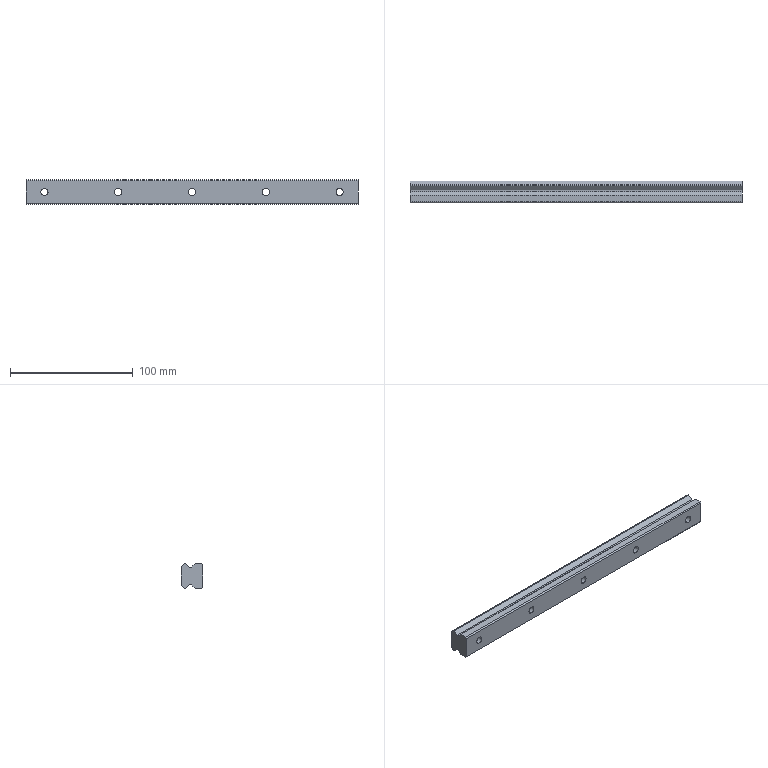Part | SolidWorks | features BaseBody 1 | 1 solid | 43 faces | box 270 x 17.5 x 20 mm | volume 81053 mm3 | plane 23 | cylinder 20 | commonest cylinder face diameters 5.8 x10 9.5 x10
STEP:
#1=CARTESIAN_POINT('',(64.75,9.,0.));
#2=VERTEX_POINT('',#1);
#3=CARTESIAN_POINT('',(55.25,9.,0.));
#4=VERTEX_POINT('',#3);
#5=CARTESIAN_POINT('',(60.,9.,0.));
#6=DIRECTION('',(0.,-1.,0.));
#7=DIRECTION('',(1.,0.,0.));
#8=AXIS2_PLACEMENT_3D('',#5,#6,#7);
#9=CIRCLE('',#8,4.75);
#10=EDGE_CURVE('',#2,#4,#9,.T.);
#11=ORIENTED_EDGE('',*,*,#10,.T.);
#12=CARTESIAN_POINT('',(55.25,17.5,0.));
#13=VERTEX_POINT('',#12);
#14=CARTESIAN_POINT('',(55.25,0.,0.));
#15=DIRECTION('',(0.,1.,0.));
#16=VECTOR('',#15,1000.);
#17=LINE('',#14,#16);
#18=EDGE_CURVE('',#4,#13,#17,.T.);
#19=ORIENTED_EDGE('',*,*,#18,.T.);
#20=CARTESIAN_POINT('',(64.75,17.5,0.));
#21=VERTEX_POINT('',#20);
#22=CARTESIAN_POINT('',(60.,17.5,0.));
#23=DIRECTION('',(0.,-1.,0.));
#24=DIRECTION('',(1.,0.,0.));
#25=AXIS2_PLACEMENT_3D('',#22,#23,#24);
#26=CIRCLE('',#25,4.75);
#27=EDGE_CURVE('',#21,#13,#26,.T.);
#28=ORIENTED_EDGE('',*,*,#27,.F.);
#29=CARTESIAN_POINT('',(64.75,0.,0.));
#30=DIRECTION('',(0.,1.,0.));
#31=VECTOR('',#30,1000.);
#32=LINE('',#29,#31);
#33=EDGE_CURVE('',#2,#21,#32,.T.);
#34=ORIENTED_EDGE('',*,*,#33,.F.);
#35=EDGE_LOOP('',(#11,#19,#28,#34));
#36=FACE_OUTER_BOUND('',#35,.T.);
#37=CARTESIAN_POINT('',(60.,0.,0.));
#38=DIRECTION('',(0.,1.,0.));
#39=DIRECTION('',(1.,0.,0.));
#40=AXIS2_PLACEMENT_3D('',#37,#38,#39);
#41=CYLINDRICAL_SURFACE('',#40,4.75);
#42=ADVANCED_FACE('',(#36),#41,.F.);
#43=CARTESIAN_POINT('',(62.9,0.,0.));
#44=VERTEX_POINT('',#43);
#45=CARTESIAN_POINT('',(57.1,0.,0.));
#46=VERTEX_POINT('',#45);
#47=CARTESIAN_POINT('',(60.,0.,0.));
#48=DIRECTION('',(0.,-1.,0.));
#49=DIRECTION('',(1.,0.,0.));
#50=AXIS2_PLACEMENT_3D('',#47,#48,#49);
#51=CIRCLE('',#50,2.9);
#52=EDGE_CURVE('',#44,#46,#51,.T.);
#53=ORIENTED_EDGE('',*,*,#52,.T.);
#54=CARTESIAN_POINT('',(57.1,9.,0.));
#55=VERTEX_POINT('',#54);
#56=CARTESIAN_POINT('',(57.1,0.,0.));
#57=DIRECTION('',(0.,1.,0.));
#58=VECTOR('',#57,1000.);
#59=LINE('',#56,#58);
#60=EDGE_CURVE('',#46,#55,#59,.T.);
#61=ORIENTED_EDGE('',*,*,#60,.T.);
#62=CARTESIAN_POINT('',(62.9,9.,0.));
#63=VERTEX_POINT('',#62);
#64=CARTESIAN_POINT('',(60.,9.,0.));
#65=DIRECTION('',(0.,-1.,0.));
#66=DIRECTION('',(1.,0.,0.));
#67=AXIS2_PLACEMENT_3D('',#64,#65,#66);
#68=CIRCLE('',#67,2.9);
#69=EDGE_CURVE('',#63,#55,#68,.T.);
#70=ORIENTED_EDGE('',*,*,#69,.F.);
#71=CARTESIAN_POINT('',(62.9,0.,0.));
#72=DIRECTION('',(0.,1.,0.));
#73=VECTOR('',#72,1000.);
#74=LINE('',#71,#73);
#75=EDGE_CURVE('',#44,#63,#74,.T.);
#76=ORIENTED_EDGE('',*,*,#75,.F.);
#77=EDGE_LOOP('',(#53,#61,#70,#76));
#78=FACE_OUTER_BOUND('',#77,.T.);
#79=CARTESIAN_POINT('',(60.,0.,0.));
#80=DIRECTION('',(0.,1.,0.));
#81=DIRECTION('',(1.,0.,0.));
#82=AXIS2_PLACEMENT_3D('',#79,#80,#81);
#83=CYLINDRICAL_SURFACE('',#82,2.9);
#84=ADVANCED_FACE('',(#78),#83,.F.);
#85=CARTESIAN_POINT('',(120.,9.,-4.75));
#86=VERTEX_POINT('',#85);
#87=CARTESIAN_POINT('',(120.,9.,4.75));
#88=VERTEX_POINT('',#87);
#89=CARTESIAN_POINT('',(120.,9.,0.));
#90=DIRECTION('',(0.,-1.,0.));
#91=DIRECTION('',(0.,0.,-1.));
#92=AXIS2_PLACEMENT_3D('',#89,#90,#91);
#93=CIRCLE('',#92,4.75);
#94=EDGE_CURVE('',#86,#88,#93,.T.);
#95=ORIENTED_EDGE('',*,*,#94,.T.);
#96=CARTESIAN_POINT('',(120.,17.5,4.75));
#97=VERTEX_POINT('',#96);
#98=CARTESIAN_POINT('',(120.,0.,4.75));
#99=DIRECTION('',(0.,1.,0.));
#100=VECTOR('',#99,1000.);
#101=LINE('',#98,#100);
#102=EDGE_CURVE('',#88,#97,#101,.T.);
#103=ORIENTED_EDGE('',*,*,#102,.T.);
#104=CARTESIAN_POINT('',(120.,17.5,-4.75));
#105=VERTEX_POINT('',#104);
#106=CARTESIAN_POINT('',(120.,17.5,0.));
#107=DIRECTION('',(0.,-1.,0.));
#108=DIRECTION('',(0.,0.,-1.));
#109=AXIS2_PLACEMENT_3D('',#106,#107,#108);
#110=CIRCLE('',#109,4.75);
#111=EDGE_CURVE('',#105,#97,#110,.T.);
#112=ORIENTED_EDGE('',*,*,#111,.F.);
#113=CARTESIAN_POINT('',(120.,0.,-4.75));
#114=DIRECTION('',(0.,1.,0.));
#115=VECTOR('',#114,1000.);
#116=LINE('',#113,#115);
#117=EDGE_CURVE('',#86,#105,#116,.T.);
#118=ORIENTED_EDGE('',*,*,#117,.F.);
#119=EDGE_LOOP('',(#95,#103,#112,#118));
#120=FACE_OUTER_BOUND('',#119,.T.);
#121=CARTESIAN_POINT('',(120.,0.,0.));
#122=DIRECTION('',(0.,1.,0.));
#123=DIRECTION('',(0.,0.,-1.));
#124=AXIS2_PLACEMENT_3D('',#121,#122,#123);
#125=CYLINDRICAL_SURFACE('',#124,4.75);
#126=ADVANCED_FACE('',(#120),#125,.F.);
#127=CARTESIAN_POINT('',(120.,0.,-2.9));
#128=VERTEX_POINT('',#127);
#129=CARTESIAN_POINT('',(120.,0.,2.9));
#130=VERTEX_POINT('',#129);
#131=CARTESIAN_POINT('',(120.,0.,0.));
#132=DIRECTION('',(0.,-1.,0.));
#133=DIRECTION('',(0.,0.,-1.));
#134=AXIS2_PLACEMENT_3D('',#131,#132,#133);
#135=CIRCLE('',#134,2.9);
#136=EDGE_CURVE('',#128,#130,#135,.T.);
#137=ORIENTED_EDGE('',*,*,#136,.T.);
#138=CARTESIAN_POINT('',(120.,9.,2.9));
#139=VERTEX_POINT('',#138);
#140=CARTESIAN_POINT('',(120.,0.,2.9));
#141=DIRECTION('',(0.,1.,0.));
#142=VECTOR('',#141,1000.);
#143=LINE('',#140,#142);
#144=EDGE_CURVE('',#130,#139,#143,.T.);
#145=ORIENTED_EDGE('',*,*,#144,.T.);
#146=CARTESIAN_POINT('',(120.,9.,-2.9));
#147=VERTEX_POINT('',#146);
#148=CARTESIAN_POINT('',(120.,9.,0.));
#149=DIRECTION('',(0.,-1.,0.));
#150=DIRECTION('',(0.,0.,-1.));
#151=AXIS2_PLACEMENT_3D('',#148,#149,#150);
#152=CIRCLE('',#151,2.9);
#153=EDGE_CURVE('',#147,#139,#152,.T.);
#154=ORIENTED_EDGE('',*,*,#153,.F.);
#155=CARTESIAN_POINT('',(120.,0.,-2.9));
#156=DIRECTION('',(0.,1.,0.));
#157=VECTOR('',#156,1000.);
#158=LINE('',#155,#157);
#159=EDGE_CURVE('',#128,#147,#158,.T.);
#160=ORIENTED_EDGE('',*,*,#159,.F.);
#161=EDGE_LOOP('',(#137,#145,#154,#160));
#162=FACE_OUTER_BOUND('',#161,.T.);
#163=CARTESIAN_POINT('',(120.,0.,0.));
#164=DIRECTION('',(0.,1.,0.));
#165=DIRECTION('',(0.,0.,-1.));
#166=AXIS2_PLACEMENT_3D('',#163,#164,#165);
#167=CYLINDRICAL_SURFACE('',#166,2.9);
#168=ADVANCED_FACE('',(#162),#167,.F.);
#169=CARTESIAN_POINT('',(180.,9.,-4.75));
#170=VERTEX_POINT('',#169);
#171=CARTESIAN_POINT('',(180.,9.,4.75));
#172=VERTEX_POINT('',#171);
#173=CARTESIAN_POINT('',(180.,9.,0.));
#174=DIRECTION('',(0.,-1.,0.));
#175=DIRECTION('',(0.,0.,-1.));
#176=AXIS2_PLACEMENT_3D('',#173,#174,#175);
#177=CIRCLE('',#176,4.75);
#178=EDGE_CURVE('',#170,#172,#177,.T.);
#179=ORIENTED_EDGE('',*,*,#178,.T.);
#180=CARTESIAN_POINT('',(180.,17.5,4.75));
#181=VERTEX_POINT('',#180);
#182=CARTESIAN_POINT('',(180.,0.,4.75));
#183=DIRECTION('',(0.,1.,0.));
#184=VECTOR('',#183,1000.);
#185=LINE('',#182,#184);
#186=EDGE_CURVE('',#172,#181,#185,.T.);
#187=ORIENTED_EDGE('',*,*,#186,.T.);
#188=CARTESIAN_POINT('',(180.,17.5,-4.75));
#189=VERTEX_POINT('',#188);
#190=CARTESIAN_POINT('',(180.,17.5,0.));
#191=DIRECTION('',(0.,-1.,0.));
#192=DIRECTION('',(0.,0.,-1.));
#193=AXIS2_PLACEMENT_3D('',#190,#191,#192);
#194=CIRCLE('',#193,4.75);
#195=EDGE_CURVE('',#189,#181,#194,.T.);
#196=ORIENTED_EDGE('',*,*,#195,.F.);
#197=CARTESIAN_POINT('',(180.,0.,-4.75));
#198=DIRECTION('',(0.,1.,0.));
#199=VECTOR('',#198,1000.);
#200=LINE('',#197,#199);
#201=EDGE_CURVE('',#170,#189,#200,.T.);
#202=ORIENTED_EDGE('',*,*,#201,.F.);
#203=EDGE_LOOP('',(#179,#187,#196,#202));
#204=FACE_OUTER_BOUND('',#203,.T.);
#205=CARTESIAN_POINT('',(180.,0.,0.));
#206=DIRECTION('',(0.,1.,0.));
#207=DIRECTION('',(0.,0.,-1.));
#208=AXIS2_PLACEMENT_3D('',#205,#206,#207);
#209=CYLINDRICAL_SURFACE('',#208,4.75);
#210=ADVANCED_FACE('',(#204),#209,.F.);
#211=CARTESIAN_POINT('',(180.,0.,-2.9));
#212=VERTEX_POINT('',#211);
#213=CARTESIAN_POINT('',(180.,0.,2.9));
#214=VERTEX_POINT('',#213);
#215=CARTESIAN_POINT('',(180.,0.,0.));
#216=DIRECTION('',(0.,-1.,0.));
#217=DIRECTION('',(0.,0.,-1.));
#218=AXIS2_PLACEMENT_3D('',#215,#216,#217);
#219=CIRCLE('',#218,2.9);
#220=EDGE_CURVE('',#212,#214,#219,.T.);
#221=ORIENTED_EDGE('',*,*,#220,.T.);
#222=CARTESIAN_POINT('',(180.,9.,2.9));
#223=VERTEX_POINT('',#222);
#224=CARTESIAN_POINT('',(180.,0.,2.9));
#225=DIRECTION('',(0.,1.,0.));
#226=VECTOR('',#225,1000.);
#227=LINE('',#224,#226);
#228=EDGE_CURVE('',#214,#223,#227,.T.);
#229=ORIENTED_EDGE('',*,*,#228,.T.);
#230=CARTESIAN_POINT('',(180.,9.,-2.9));
#231=VERTEX_POINT('',#230);
#232=CARTESIAN_POINT('',(180.,9.,0.));
#233=DIRECTION('',(0.,-1.,0.));
#234=DIRECTION('',(0.,0.,-1.));
#235=AXIS2_PLACEMENT_3D('',#232,#233,#234);
#236=CIRCLE('',#235,2.9);
#237=EDGE_CURVE('',#231,#223,#236,.T.);
#238=ORIENTED_EDGE('',*,*,#237,.F.);
#239=CARTESIAN_POINT('',(180.,0.,-2.9));
#240=DIRECTION('',(0.,1.,0.));
#241=VECTOR('',#240,1000.);
#242=LINE('',#239,#241);
#243=EDGE_CURVE('',#212,#231,#242,.T.);
#244=ORIENTED_EDGE('',*,*,#243,.F.);
#245=EDGE_LOOP('',(#221,#229,#238,#244));
#246=FACE_OUTER_BOUND('',#245,.T.);
#247=CARTESIAN_POINT('',(180.,0.,0.));
#248=DIRECTION('',(0.,1.,0.));
#249=DIRECTION('',(0.,0.,-1.));
#250=AXIS2_PLACEMENT_3D('',#247,#248,#249);
#251=CYLINDRICAL_SURFACE('',#250,2.9);
#252=ADVANCED_FACE('',(#246),#251,.F.);
#253=CARTESIAN_POINT('',(240.,9.,-4.75));
#254=VERTEX_POINT('',#253);
#255=CARTESIAN_POINT('',(240.,9.,4.75));
#256=VERTEX_POINT('',#255);
#257=CARTESIAN_POINT('',(240.,9.,0.));
#258=DIRECTION('',(0.,-1.,0.));
#259=DIRECTION('',(0.,0.,-1.));
#260=AXIS2_PLACEMENT_3D('',#257,#258,#259);
#261=CIRCLE('',#260,4.75);
#262=EDGE_CURVE('',#254,#256,#261,.T.);
#263=ORIENTED_EDGE('',*,*,#262,.T.);
#264=CARTESIAN_POINT('',(240.,17.5,4.75));
#265=VERTEX_POINT('',#264);
#266=CARTESIAN_POINT('',(240.,0.,4.75));
#267=DIRECTION('',(0.,1.,0.));
#268=VECTOR('',#267,1000.);
#269=LINE('',#266,#268);
#270=EDGE_CURVE('',#256,#265,#269,.T.);
#271=ORIENTED_EDGE('',*,*,#270,.T.);
#272=CARTESIAN_POINT('',(240.,17.5,-4.75));
#273=VERTEX_POINT('',#272);
#274=CARTESIAN_POINT('',(240.,17.5,0.));
#275=DIRECTION('',(0.,-1.,0.));
#276=DIRECTION('',(0.,0.,-1.));
#277=AXIS2_PLACEMENT_3D('',#274,#275,#276);
#278=CIRCLE('',#277,4.75);
#279=EDGE_CURVE('',#273,#265,#278,.T.);
#280=ORIENTED_EDGE('',*,*,#279,.F.);
#281=CARTESIAN_POINT('',(240.,0.,-4.75));
#282=DIRECTION('',(0.,1.,0.));
#283=VECTOR('',#282,1000.);
#284=LINE('',#281,#283);
#285=EDGE_CURVE('',#254,#273,#284,.T.);
#286=ORIENTED_EDGE('',*,*,#285,.F.);
#287=EDGE_LOOP('',(#263,#271,#280,#286));
#288=FACE_OUTER_BOUND('',#287,.T.);
#289=CARTESIAN_POINT('',(240.,0.,0.));
#290=DIRECTION('',(0.,1.,0.));
#291=DIRECTION('',(0.,0.,-1.));
#292=AXIS2_PLACEMENT_3D('',#289,#290,#291);
#293=CYLINDRICAL_SURFACE('',#292,4.75);
#294=ADVANCED_FACE('',(#288),#293,.F.);
#295=CARTESIAN_POINT('',(240.,0.,-2.9));
#296=VERTEX_POINT('',#295);
#297=CARTESIAN_POINT('',(240.,0.,2.9));
#298=VERTEX_POINT('',#297);
#299=CARTESIAN_POINT('',(240.,0.,0.));
#300=DIRECTION('',(0.,-1.,0.));
#301=DIRECTION('',(0.,0.,-1.));
#302=AXIS2_PLACEMENT_3D('',#299,#300,#301);
#303=CIRCLE('',#302,2.9);
#304=EDGE_CURVE('',#296,#298,#303,.T.);
#305=ORIENTED_EDGE('',*,*,#304,.T.);
#306=CARTESIAN_POINT('',(240.,9.,2.9));
#307=VERTEX_POINT('',#306);
#308=CARTESIAN_POINT('',(240.,0.,2.9));
#309=DIRECTION('',(0.,1.,0.));
#310=VECTOR('',#309,1000.);
#311=LINE('',#308,#310);
#312=EDGE_CURVE('',#298,#307,#311,.T.);
#313=ORIENTED_EDGE('',*,*,#312,.T.);
#314=CARTESIAN_POINT('',(240.,9.,-2.9));
#315=VERTEX_POINT('',#314);
#316=CARTESIAN_POINT('',(240.,9.,0.));
#317=DIRECTION('',(0.,-1.,0.));
#318=DIRECTION('',(0.,0.,-1.));
#319=AXIS2_PLACEMENT_3D('',#316,#317,#318);
#320=CIRCLE('',#319,2.9);
#321=EDGE_CURVE('',#315,#307,#320,.T.);
#322=ORIENTED_EDGE('',*,*,#321,.F.);
#323=CARTESIAN_POINT('',(240.,0.,-2.9));
#324=DIRECTION('',(0.,1.,0.));
#325=VECTOR('',#324,1000.);
#326=LINE('',#323,#325);
#327=EDGE_CURVE('',#296,#315,#326,.T.);
#328=ORIENTED_EDGE('',*,*,#327,.F.);
#329=EDGE_LOOP('',(#305,#313,#322,#328));
#330=FACE_OUTER_BOUND('',#329,.T.);
#331=CARTESIAN_POINT('',(240.,0.,0.));
#332=DIRECTION('',(0.,1.,0.));
#333=DIRECTION('',(0.,0.,-1.));
#334=AXIS2_PLACEMENT_3D('',#331,#332,#333);
#335=CYLINDRICAL_SURFACE('',#334,2.9);
#336=ADVANCED_FACE('',(#330),#335,.F.);
#337=CARTESIAN_POINT('',(300.,9.,-4.75));
#338=VERTEX_POINT('',#337);
#339=CARTESIAN_POINT('',(300.,9.,4.75));
#340=VERTEX_POINT('',#339);
#341=CARTESIAN_POINT('',(300.,9.,0.));
#342=DIRECTION('',(0.,-1.,0.));
#343=DIRECTION('',(0.,0.,-1.));
#344=AXIS2_PLACEMENT_3D('',#341,#342,#343);
#345=CIRCLE('',#344,4.75);
#346=EDGE_CURVE('',#338,#340,#345,.T.);
#347=ORIENTED_EDGE('',*,*,#346,.T.);
#348=CARTESIAN_POINT('',(300.,17.5,4.75));
#349=VERTEX_POINT('',#348);
#350=CARTESIAN_POINT('',(300.,0.,4.75));
#351=DIRECTION('',(0.,1.,0.));
#352=VECTOR('',#351,1000.);
#353=LINE('',#350,#352);
#354=EDGE_CURVE('',#340,#349,#353,.T.);
#355=ORIENTED_EDGE('',*,*,#354,.T.);
#356=CARTESIAN_POINT('',(300.,17.5,-4.75));
#357=VERTEX_POINT('',#356);
#358=CARTESIAN_POINT('',(300.,17.5,0.));
#359=DIRECTION('',(0.,-1.,0.));
#360=DIRECTION('',(0.,0.,-1.));
#361=AXIS2_PLACEMENT_3D('',#358,#359,#360);
#362=CIRCLE('',#361,4.75);
#363=EDGE_CURVE('',#357,#349,#362,.T.);
#364=ORIENTED_EDGE('',*,*,#363,.F.);
#365=CARTESIAN_POINT('',(300.,0.,-4.75));
#366=DIRECTION('',(0.,1.,0.));
#367=VECTOR('',#366,1000.);
#368=LINE('',#365,#367);
#369=EDGE_CURVE('',#338,#357,#368,.T.);
#370=ORIENTED_EDGE('',*,*,#369,.F.);
#371=EDGE_LOOP('',(#347,#355,#364,#370));
#372=FACE_OUTER_BOUND('',#371,.T.);
#373=CARTESIAN_POINT('',(300.,0.,0.));
#374=DIRECTION('',(0.,1.,0.));
#375=DIRECTION('',(0.,0.,-1.));
#376=AXIS2_PLACEMENT_3D('',#373,#374,#375);
#377=CYLINDRICAL_SURFACE('',#376,4.75);
#378=ADVANCED_FACE('',(#372),#377,.F.);
#379=CARTESIAN_POINT('',(300.,0.,-2.9));
#380=VERTEX_POINT('',#379);
#381=CARTESIAN_POINT('',(300.,0.,2.9));
#382=VERTEX_POINT('',#381);
#383=CARTESIAN_POINT('',(300.,0.,0.));
#384=DIRECTION('',(0.,-1.,0.));
#385=DIRECTION('',(0.,0.,-1.));
#386=AXIS2_PLACEMENT_3D('',#383,#384,#385);
#387=CIRCLE('',#386,2.9);
#388=EDGE_CURVE('',#380,#382,#387,.T.);
#389=ORIENTED_EDGE('',*,*,#388,.T.);
#390=CARTESIAN_POINT('',(300.,9.,2.9));
#391=VERTEX_POINT('',#390);
#392=CARTESIAN_POINT('',(300.,0.,2.9));
#393=DIRECTION('',(0.,1.,0.));
#394=VECTOR('',#393,1000.);
#395=LINE('',#392,#394);
#396=EDGE_CURVE('',#382,#391,#395,.T.);
#397=ORIENTED_EDGE('',*,*,#396,.T.);
#398=CARTESIAN_POINT('',(300.,9.,-2.9));
#399=VERTEX_POINT('',#398);
#400=CARTESIAN_POINT('',(300.,9.,0.));
#401=DIRECTION('',(0.,-1.,0.));
#402=DIRECTION('',(0.,0.,-1.));
#403=AXIS2_PLACEMENT_3D('',#400,#401,#402);
#404=CIRCLE('',#403,2.9);
#405=EDGE_CURVE('',#399,#391,#404,.T.);
#406=ORIENTED_EDGE('',*,*,#405,.F.);
#407=CARTESIAN_POINT('',(300.,0.,-2.9));
#408=DIRECTION('',(0.,1.,0.));
#409=VECTOR('',#408,1000.);
#410=LINE('',#407,#409);
#411=EDGE_CURVE('',#380,#399,#410,.T.);
#412=ORIENTED_EDGE('',*,*,#411,.F.);
#413=EDGE_LOOP('',(#389,#397,#406,#412));
#414=FACE_OUTER_BOUND('',#413,.T.);
#415=CARTESIAN_POINT('',(300.,0.,0.));
#416=DIRECTION('',(0.,1.,0.));
#417=DIRECTION('',(0.,0.,-1.));
#418=AXIS2_PLACEMENT_3D('',#415,#416,#417);
#419=CYLINDRICAL_SURFACE('',#418,2.9);
#420=ADVANCED_FACE('',(#414),#419,.F.);
#421=CARTESIAN_POINT('',(45.,14.7,10.));
#422=VERTEX_POINT('',#421);
#423=CARTESIAN_POINT('',(45.,17.5,7.37));
#424=VERTEX_POINT('',#423);
#425=CARTESIAN_POINT('',(45.,17.5,7.37));
#426=DIRECTION('',(0.,0.7289,-0.6846));
#427=VECTOR('',#426,1000.);
#428=LINE('',#425,#427);
#429=EDGE_CURVE('',#422,#424,#428,.T.);
#430=ORIENTED_EDGE('',*,*,#429,.T.);
#431=CARTESIAN_POINT('',(45.,17.5,-7.37));
#432=VERTEX_POINT('',#431);
#433=CARTESIAN_POINT('',(45.,17.5,-40.));
#434=DIRECTION('',(0.,0.,1.));
#435=VECTOR('',#434,1000.);
#436=LINE('',#433,#435);
#437=EDGE_CURVE('',#432,#424,#436,.T.);
#438=ORIENTED_EDGE('',*,*,#437,.F.);
#439=CARTESIAN_POINT('',(45.,14.7,-10.));
#440=VERTEX_POINT('',#439);
#441=CARTESIAN_POINT('',(45.,14.7,-10.));
#442=DIRECTION('',(0.,-0.7289,-0.6846));
#443=VECTOR('',#442,1000.);
#444=LINE('',#441,#443);
#445=EDGE_CURVE('',#432,#440,#444,.T.);
#446=ORIENTED_EDGE('',*,*,#445,.T.);
#447=CARTESIAN_POINT('',(45.,13.86,-10.));
#448=VERTEX_POINT('',#447);
#449=CARTESIAN_POINT('',(45.,13.86,-10.));
#450=DIRECTION('',(0.,-1.,0.));
#451=VECTOR('',#450,1000.);
#452=LINE('',#449,#451);
#453=EDGE_CURVE('',#440,#448,#452,.T.);
#454=ORIENTED_EDGE('',*,*,#453,.T.);
#455=CARTESIAN_POINT('',(45.,10.6,-7.25));
#456=VERTEX_POINT('',#455);
#457=CARTESIAN_POINT('',(45.,10.6,-7.25));
#458=DIRECTION('',(0.,-0.7644,0.6448));
#459=VECTOR('',#458,1000.);
#460=LINE('',#457,#459);
#461=EDGE_CURVE('',#448,#456,#460,.T.);
#462=ORIENTED_EDGE('',*,*,#461,.T.);
#463=CARTESIAN_POINT('',(45.,8.9,-7.25));
#464=VERTEX_POINT('',#463);
#465=CARTESIAN_POINT('',(45.,8.9,-7.25));
#466=DIRECTION('',(0.,-1.,0.));
#467=VECTOR('',#466,1000.);
#468=LINE('',#465,#467);
#469=EDGE_CURVE('',#456,#464,#468,.T.);
#470=ORIENTED_EDGE('',*,*,#469,.T.);
#471=CARTESIAN_POINT('',(45.,6.15,-10.));
#472=VERTEX_POINT('',#471);
#473=CARTESIAN_POINT('',(45.,6.15,-10.));
#474=DIRECTION('',(0.,-0.7071,-0.7071));
#475=VECTOR('',#474,1000.);
#476=LINE('',#473,#475);
#477=EDGE_CURVE('',#464,#472,#476,.T.);
#478=ORIENTED_EDGE('',*,*,#477,.T.);
#479=CARTESIAN_POINT('',(45.,1.,-10.));
#480=VERTEX_POINT('',#479);
#481=CARTESIAN_POINT('',(45.,1.,-10.));
#482=DIRECTION('',(0.,-1.,0.));
#483=VECTOR('',#482,1000.);
#484=LINE('',#481,#483);
#485=EDGE_CURVE('',#472,#480,#484,.T.);
#486=ORIENTED_EDGE('',*,*,#485,.T.);
#487=CARTESIAN_POINT('',(45.,0.,-9.));
#488=VERTEX_POINT('',#487);
#489=CARTESIAN_POINT('',(45.,0.,-9.));
#490=DIRECTION('',(0.,-0.7071,0.7071));
#491=VECTOR('',#490,1000.);
#492=LINE('',#489,#491);
#493=EDGE_CURVE('',#480,#488,#492,.T.);
#494=ORIENTED_EDGE('',*,*,#493,.T.);
#495=CARTESIAN_POINT('',(45.,0.,9.));
#496=VERTEX_POINT('',#495);
#497=CARTESIAN_POINT('',(45.,0.,9.));
#498=DIRECTION('',(0.,0.,1.));
#499=VECTOR('',#498,1000.);
#500=LINE('',#497,#499);
#501=EDGE_CURVE('',#488,#496,#500,.T.);
#502=ORIENTED_EDGE('',*,*,#501,.T.);
#503=CARTESIAN_POINT('',(45.,1.,10.));
#504=VERTEX_POINT('',#503);
#505=CARTESIAN_POINT('',(45.,1.,10.));
#506=DIRECTION('',(0.,0.7071,0.7071));
#507=VECTOR('',#506,1000.);
#508=LINE('',#505,#507);
#509=EDGE_CURVE('',#496,#504,#508,.T.);
#510=ORIENTED_EDGE('',*,*,#509,.T.);
#511=CARTESIAN_POINT('',(45.,6.15,10.));
#512=VERTEX_POINT('',#511);
#513=CARTESIAN_POINT('',(45.,6.15,10.));
#514=DIRECTION('',(0.,1.,0.));
#515=VECTOR('',#514,1000.);
#516=LINE('',#513,#515);
#517=EDGE_CURVE('',#504,#512,#516,.T.);
#518=ORIENTED_EDGE('',*,*,#517,.T.);
#519=CARTESIAN_POINT('',(45.,8.9,7.25));
#520=VERTEX_POINT('',#519);
#521=CARTESIAN_POINT('',(45.,8.9,7.25));
#522=DIRECTION('',(0.,0.7071,-0.7071));
#523=VECTOR('',#522,1000.);
#524=LINE('',#521,#523);
#525=EDGE_CURVE('',#512,#520,#524,.T.);
#526=ORIENTED_EDGE('',*,*,#525,.T.);
#527=CARTESIAN_POINT('',(45.,10.6,7.25));
#528=VERTEX_POINT('',#527);
#529=CARTESIAN_POINT('',(45.,10.6,7.25));
#530=DIRECTION('',(0.,1.,0.));
#531=VECTOR('',#530,1000.);
#532=LINE('',#529,#531);
#533=EDGE_CURVE('',#520,#528,#532,.T.);
#534=ORIENTED_EDGE('',*,*,#533,.T.);
#535=CARTESIAN_POINT('',(45.,13.86,10.));
#536=VERTEX_POINT('',#535);
#537=CARTESIAN_POINT('',(45.,13.86,10.));
#538=DIRECTION('',(0.,0.7644,0.6448));
#539=VECTOR('',#538,1000.);
#540=LINE('',#537,#539);
#541=EDGE_CURVE('',#528,#536,#540,.T.);
#542=ORIENTED_EDGE('',*,*,#541,.T.);
#543=CARTESIAN_POINT('',(45.,14.7,10.));
#544=DIRECTION('',(0.,1.,0.));
#545=VECTOR('',#544,1000.);
#546=LINE('',#543,#545);
#547=EDGE_CURVE('',#536,#422,#546,.T.);
#548=ORIENTED_EDGE('',*,*,#547,.T.);
#549=EDGE_LOOP('',(#430,#438,#446,#454,#462,#470,#478,#486,#494,#502,#510,#518,#526,#534,#542,#548));
#550=FACE_OUTER_BOUND('',#549,.T.);
#551=CARTESIAN_POINT('',(45.,-32.5,-40.));
#552=DIRECTION('',(-1.,0.,0.));
#553=DIRECTION('',(0.,0.,1.));
#554=AXIS2_PLACEMENT_3D('',#551,#552,#553);
#555=PLANE('',#554);
#556=ADVANCED_FACE('',(#550),#555,.T.);
#557=CARTESIAN_POINT('',(315.,17.5,7.37));
#558=VERTEX_POINT('',#557);
#559=CARTESIAN_POINT('',(315.,14.7,10.));
#560=VERTEX_POINT('',#559);
#561=CARTESIAN_POINT('',(315.,17.5,7.37));
#562=DIRECTION('',(0.,-0.7289,0.6846));
#563=VECTOR('',#562,1000.);
#564=LINE('',#561,#563);
#565=EDGE_CURVE('',#558,#560,#564,.T.);
#566=ORIENTED_EDGE('',*,*,#565,.T.);
#567=CARTESIAN_POINT('',(315.,13.86,10.));
#568=VERTEX_POINT('',#567);
#569=CARTESIAN_POINT('',(315.,14.7,10.));
#570=DIRECTION('',(0.,-1.,0.));
#571=VECTOR('',#570,1000.);
#572=LINE('',#569,#571);
#573=EDGE_CURVE('',#560,#568,#572,.T.);
#574=ORIENTED_EDGE('',*,*,#573,.T.);
#575=CARTESIAN_POINT('',(315.,10.6,7.25));
#576=VERTEX_POINT('',#575);
#577=CARTESIAN_POINT('',(315.,13.86,10.));
#578=DIRECTION('',(0.,-0.7644,-0.6448));
#579=VECTOR('',#578,1000.);
#580=LINE('',#577,#579);
#581=EDGE_CURVE('',#568,#576,#580,.T.);
#582=ORIENTED_EDGE('',*,*,#581,.T.);
#583=CARTESIAN_POINT('',(315.,8.9,7.25));
#584=VERTEX_POINT('',#583);
#585=CARTESIAN_POINT('',(315.,10.6,7.25));
#586=DIRECTION('',(0.,-1.,0.));
#587=VECTOR('',#586,1000.);
#588=LINE('',#585,#587);
#589=EDGE_CURVE('',#576,#584,#588,.T.);
#590=ORIENTED_EDGE('',*,*,#589,.T.);
#591=CARTESIAN_POINT('',(315.,6.15,10.));
#592=VERTEX_POINT('',#591);
#593=CARTESIAN_POINT('',(315.,8.9,7.25));
#594=DIRECTION('',(0.,-0.7071,0.7071));
#595=VECTOR('',#594,1000.);
#596=LINE('',#593,#595);
#597=EDGE_CURVE('',#584,#592,#596,.T.);
#598=ORIENTED_EDGE('',*,*,#597,.T.);
#599=CARTESIAN_POINT('',(315.,1.,10.));
#600=VERTEX_POINT('',#599);
#601=CARTESIAN_POINT('',(315.,6.15,10.));
#602=DIRECTION('',(0.,-1.,0.));
#603=VECTOR('',#602,1000.);
#604=LINE('',#601,#603);
#605=EDGE_CURVE('',#592,#600,#604,.T.);
#606=ORIENTED_EDGE('',*,*,#605,.T.);
#607=CARTESIAN_POINT('',(315.,0.,9.));
#608=VERTEX_POINT('',#607);
#609=CARTESIAN_POINT('',(315.,1.,10.));
#610=DIRECTION('',(0.,-0.7071,-0.7071));
#611=VECTOR('',#610,1000.);
#612=LINE('',#609,#611);
#613=EDGE_CURVE('',#600,#608,#612,.T.);
#614=ORIENTED_EDGE('',*,*,#613,.T.);
#615=CARTESIAN_POINT('',(315.,0.,-9.));
#616=VERTEX_POINT('',#615);
#617=CARTESIAN_POINT('',(315.,0.,9.));
#618=DIRECTION('',(0.,0.,-1.));
#619=VECTOR('',#618,1000.);
#620=LINE('',#617,#619);
#621=EDGE_CURVE('',#608,#616,#620,.T.);
#622=ORIENTED_EDGE('',*,*,#621,.T.);
#623=CARTESIAN_POINT('',(315.,1.,-10.));
#624=VERTEX_POINT('',#623);
#625=CARTESIAN_POINT('',(315.,0.,-9.));
#626=DIRECTION('',(0.,0.7071,-0.7071));
#627=VECTOR('',#626,1000.);
#628=LINE('',#625,#627);
#629=EDGE_CURVE('',#616,#624,#628,.T.);
#630=ORIENTED_EDGE('',*,*,#629,.T.);
#631=CARTESIAN_POINT('',(315.,6.15,-10.));
#632=VERTEX_POINT('',#631);
#633=CARTESIAN_POINT('',(315.,1.,-10.));
#634=DIRECTION('',(0.,1.,0.));
#635=VECTOR('',#634,1000.);
#636=LINE('',#633,#635);
#637=EDGE_CURVE('',#624,#632,#636,.T.);
#638=ORIENTED_EDGE('',*,*,#637,.T.);
#639=CARTESIAN_POINT('',(315.,8.9,-7.25));
#640=VERTEX_POINT('',#639);
#641=CARTESIAN_POINT('',(315.,6.15,-10.));
#642=DIRECTION('',(0.,0.7071,0.7071));
#643=VECTOR('',#642,1000.);
#644=LINE('',#641,#643);
#645=EDGE_CURVE('',#632,#640,#644,.T.);
#646=ORIENTED_EDGE('',*,*,#645,.T.);
#647=CARTESIAN_POINT('',(315.,10.6,-7.25));
#648=VERTEX_POINT('',#647);
#649=CARTESIAN_POINT('',(315.,8.9,-7.25));
#650=DIRECTION('',(0.,1.,0.));
#651=VECTOR('',#650,1000.);
#652=LINE('',#649,#651);
#653=EDGE_CURVE('',#640,#648,#652,.T.);
#654=ORIENTED_EDGE('',*,*,#653,.T.);
#655=CARTESIAN_POINT('',(315.,13.86,-10.));
#656=VERTEX_POINT('',#655);
#657=CARTESIAN_POINT('',(315.,10.6,-7.25));
#658=DIRECTION('',(0.,0.7644,-0.6448));
#659=VECTOR('',#658,1000.);
#660=LINE('',#657,#659);
#661=EDGE_CURVE('',#648,#656,#660,.T.);
#662=ORIENTED_EDGE('',*,*,#661,.T.);
#663=CARTESIAN_POINT('',(315.,14.7,-10.));
#664=VERTEX_POINT('',#663);
#665=CARTESIAN_POINT('',(315.,13.86,-10.));
#666=DIRECTION('',(0.,1.,0.));
#667=VECTOR('',#666,1000.);
#668=LINE('',#665,#667);
#669=EDGE_CURVE('',#656,#664,#668,.T.);
#670=ORIENTED_EDGE('',*,*,#669,.T.);
#671=CARTESIAN_POINT('',(315.,17.5,-7.37));
#672=VERTEX_POINT('',#671);
#673=CARTESIAN_POINT('',(315.,14.7,-10.));
#674=DIRECTION('',(0.,0.7289,0.6846));
#675=VECTOR('',#674,1000.);
#676=LINE('',#673,#675);
#677=EDGE_CURVE('',#664,#672,#676,.T.);
#678=ORIENTED_EDGE('',*,*,#677,.T.);
#679=CARTESIAN_POINT('',(315.,17.5,-40.));
#680=DIRECTION('',(0.,0.,-1.));
#681=VECTOR('',#680,1000.);
#682=LINE('',#679,#681);
#683=EDGE_CURVE('',#558,#672,#682,.T.);
#684=ORIENTED_EDGE('',*,*,#683,.F.);
#685=EDGE_LOOP('',(#566,#574,#582,#590,#598,#606,#614,#622,#630,#638,#646,#654,#662,#670,#678,#684));
#686=FACE_OUTER_BOUND('',#685,.T.);
#687=CARTESIAN_POINT('',(315.,-32.5,-40.));
#688=DIRECTION('',(1.,0.,0.));
#689=DIRECTION('',(0.,1.,0.));
#690=AXIS2_PLACEMENT_3D('',#687,#688,#689);
#691=PLANE('',#690);
#692=ADVANCED_FACE('',(#686),#691,.T.);
#693=ORIENTED_EDGE('',*,*,#69,.T.);
#694=CARTESIAN_POINT('',(60.,9.,0.));
#695=DIRECTION('',(0.,-1.,0.));
#696=DIRECTION('',(1.,0.,0.));
#697=AXIS2_PLACEMENT_3D('',#694,#695,#696);
#698=CIRCLE('',#697,2.9);
#699=EDGE_CURVE('',#55,#63,#698,.T.);
#700=ORIENTED_EDGE('',*,*,#699,.T.);
#701=EDGE_LOOP('',(#693,#700));
#702=FACE_BOUND('',#701,.T.);
#703=ORIENTED_EDGE('',*,*,#10,.F.);
#704=CARTESIAN_POINT('',(60.,9.,0.));
#705=DIRECTION('',(0.,-1.,0.));
#706=DIRECTION('',(1.,0.,0.));
#707=AXIS2_PLACEMENT_3D('',#704,#705,#706);
#708=CIRCLE('',#707,4.75);
#709=EDGE_CURVE('',#4,#2,#708,.T.);
#710=ORIENTED_EDGE('',*,*,#709,.F.);
#711=EDGE_LOOP('',(#703,#710));
#712=FACE_OUTER_BOUND('',#711,.T.);
#713=CARTESIAN_POINT('',(64.75,9.,0.));
#714=DIRECTION('',(0.,1.,0.));
#715=DIRECTION('',(1.,0.,0.));
#716=AXIS2_PLACEMENT_3D('',#713,#714,#715);
#717=PLANE('',#716);
#718=ADVANCED_FACE('',(#702,#712),#717,.T.);
#719=ORIENTED_EDGE('',*,*,#153,.T.);
#720=CARTESIAN_POINT('',(120.,9.,0.));
#721=DIRECTION('',(0.,-1.,0.));
#722=DIRECTION('',(0.,0.,-1.));
#723=AXIS2_PLACEMENT_3D('',#720,#721,#722);
#724=CIRCLE('',#723,2.9);
#725=EDGE_CURVE('',#139,#147,#724,.T.);
#726=ORIENTED_EDGE('',*,*,#725,.T.);
#727=EDGE_LOOP('',(#719,#726));
#728=FACE_BOUND('',#727,.T.);
#729=ORIENTED_EDGE('',*,*,#94,.F.);
#730=CARTESIAN_POINT('',(120.,9.,0.));
#731=DIRECTION('',(0.,-1.,0.));
#732=DIRECTION('',(0.,0.,-1.));
#733=AXIS2_PLACEMENT_3D('',#730,#731,#732);
#734=CIRCLE('',#733,4.75);
#735=EDGE_CURVE('',#88,#86,#734,.T.);
#736=ORIENTED_EDGE('',*,*,#735,.F.);
#737=EDGE_LOOP('',(#729,#736));
#738=FACE_OUTER_BOUND('',#737,.T.);
#739=CARTESIAN_POINT('',(124.75,9.,0.));
#740=DIRECTION('',(0.,1.,0.));
#741=DIRECTION('',(1.,0.,0.));
#742=AXIS2_PLACEMENT_3D('',#739,#740,#741);
#743=PLANE('',#742);
#744=ADVANCED_FACE('',(#728,#738),#743,.T.);
#745=ORIENTED_EDGE('',*,*,#237,.T.);
#746=CARTESIAN_POINT('',(180.,9.,0.));
#747=DIRECTION('',(0.,-1.,0.));
#748=DIRECTION('',(0.,0.,-1.));
#749=AXIS2_PLACEMENT_3D('',#746,#747,#748);
#750=CIRCLE('',#749,2.9);
#751=EDGE_CURVE('',#223,#231,#750,.T.);
#752=ORIENTED_EDGE('',*,*,#751,.T.);
#753=EDGE_LOOP('',(#745,#752));
#754=FACE_BOUND('',#753,.T.);
#755=ORIENTED_EDGE('',*,*,#178,.F.);
#756=CARTESIAN_POINT('',(180.,9.,0.));
#757=DIRECTION('',(0.,-1.,0.));
#758=DIRECTION('',(0.,0.,-1.));
#759=AXIS2_PLACEMENT_3D('',#756,#757,#758);
#760=CIRCLE('',#759,4.75);
#761=EDGE_CURVE('',#172,#170,#760,.T.);
#762=ORIENTED_EDGE('',*,*,#761,.F.);
#763=EDGE_LOOP('',(#755,#762));
#764=FACE_OUTER_BOUND('',#763,.T.);
#765=CARTESIAN_POINT('',(184.75,9.,0.));
#766=DIRECTION('',(0.,1.,0.));
#767=DIRECTION('',(1.,0.,0.));
#768=AXIS2_PLACEMENT_3D('',#765,#766,#767);
#769=PLANE('',#768);
#770=ADVANCED_FACE('',(#754,#764),#769,.T.);
#771=ORIENTED_EDGE('',*,*,#321,.T.);
#772=CARTESIAN_POINT('',(240.,9.,0.));
#773=DIRECTION('',(0.,-1.,0.));
#774=DIRECTION('',(0.,0.,-1.));
#775=AXIS2_PLACEMENT_3D('',#772,#773,#774);
#776=CIRCLE('',#775,2.9);
#777=EDGE_CURVE('',#307,#315,#776,.T.);
#778=ORIENTED_EDGE('',*,*,#777,.T.);
#779=EDGE_LOOP('',(#771,#778));
#780=FACE_BOUND('',#779,.T.);
#781=ORIENTED_EDGE('',*,*,#262,.F.);
#782=CARTESIAN_POINT('',(240.,9.,0.));
#783=DIRECTION('',(0.,-1.,0.));
#784=DIRECTION('',(0.,0.,-1.));
#785=AXIS2_PLACEMENT_3D('',#782,#783,#784);
#786=CIRCLE('',#785,4.75);
#787=EDGE_CURVE('',#256,#254,#786,.T.);
#788=ORIENTED_EDGE('',*,*,#787,.F.);
#789=EDGE_LOOP('',(#781,#788));
#790=FACE_OUTER_BOUND('',#789,.T.);
#791=CARTESIAN_POINT('',(244.75,9.,0.));
#792=DIRECTION('',(0.,1.,0.));
#793=DIRECTION('',(1.,0.,0.));
#794=AXIS2_PLACEMENT_3D('',#791,#792,#793);
#795=PLANE('',#794);
#796=ADVANCED_FACE('',(#780,#790),#795,.T.);
#797=ORIENTED_EDGE('',*,*,#405,.T.);
#798=CARTESIAN_POINT('',(300.,9.,0.));
#799=DIRECTION('',(0.,-1.,0.));
#800=DIRECTION('',(0.,0.,-1.));
#801=AXIS2_PLACEMENT_3D('',#798,#799,#800);
#802=CIRCLE('',#801,2.9);
#803=EDGE_CURVE('',#391,#399,#802,.T.);
#804=ORIENTED_EDGE('',*,*,#803,.T.);
#805=EDGE_LOOP('',(#797,#804));
#806=FACE_BOUND('',#805,.T.);
#807=ORIENTED_EDGE('',*,*,#346,.F.);
#808=CARTESIAN_POINT('',(300.,9.,0.));
#809=DIRECTION('',(0.,-1.,0.));
#810=DIRECTION('',(0.,0.,-1.));
#811=AXIS2_PLACEMENT_3D('',#808,#809,#810);
#812=CIRCLE('',#811,4.75);
#813=EDGE_CURVE('',#340,#338,#812,.T.);
#814=ORIENTED_EDGE('',*,*,#813,.F.);
#815=EDGE_LOOP('',(#807,#814));
#816=FACE_OUTER_BOUND('',#815,.T.);
#817=CARTESIAN_POINT('',(304.75,9.,0.));
#818=DIRECTION('',(0.,1.,0.));
#819=DIRECTION('',(1.,0.,0.));
#820=AXIS2_PLACEMENT_3D('',#817,#818,#819);
#821=PLANE('',#820);
#822=ADVANCED_FACE('',(#806,#816),#821,.T.);
#823=ORIENTED_EDGE('',*,*,#469,.F.);
#824=CARTESIAN_POINT('',(2400.,10.6,-7.25));
#825=DIRECTION('',(-1.,0.,0.));
#826=VECTOR('',#825,1000.);
#827=LINE('',#824,#826);
#828=EDGE_CURVE('',#648,#456,#827,.T.);
#829=ORIENTED_EDGE('',*,*,#828,.F.);
#830=ORIENTED_EDGE('',*,*,#653,.F.);
#831=CARTESIAN_POINT('',(2400.,8.9,-7.25));
#832=DIRECTION('',(-1.,0.,0.));
#833=VECTOR('',#832,1000.);
#834=LINE('',#831,#833);
#835=EDGE_CURVE('',#640,#464,#834,.T.);
#836=ORIENTED_EDGE('',*,*,#835,.T.);
#837=EDGE_LOOP('',(#823,#829,#830,#836));
#838=FACE_OUTER_BOUND('',#837,.T.);
#839=CARTESIAN_POINT('',(2400.,8.9,-7.25));
#840=DIRECTION('',(0.,0.,1.));
#841=DIRECTION('',(1.,0.,0.));
#842=AXIS2_PLACEMENT_3D('',#839,#840,#841);
#843=PLANE('',#842);
#844=ADVANCED_FACE('',(#838),#843,.F.);
#845=ORIENTED_EDGE('',*,*,#461,.F.);
#846=CARTESIAN_POINT('',(2400.,13.86,-10.));
#847=DIRECTION('',(-1.,0.,0.));
#848=VECTOR('',#847,1000.);
#849=LINE('',#846,#848);
#850=EDGE_CURVE('',#656,#448,#849,.T.);
#851=ORIENTED_EDGE('',*,*,#850,.F.);
#852=ORIENTED_EDGE('',*,*,#661,.F.);
#853=ORIENTED_EDGE('',*,*,#828,.T.);
#854=EDGE_LOOP('',(#845,#851,#852,#853));
#855=FACE_OUTER_BOUND('',#854,.T.);
#856=CARTESIAN_POINT('',(2400.,10.6,-7.25));
#857=DIRECTION('',(0.,0.6448,0.7644));
#858=DIRECTION('',(1.,0.,0.));
#859=AXIS2_PLACEMENT_3D('',#856,#857,#858);
#860=PLANE('',#859);
#861=ADVANCED_FACE('',(#855),#860,.F.);
#862=ORIENTED_EDGE('',*,*,#477,.F.);
#863=ORIENTED_EDGE('',*,*,#835,.F.);
#864=ORIENTED_EDGE('',*,*,#645,.F.);
#865=CARTESIAN_POINT('',(2400.,6.15,-10.));
#866=DIRECTION('',(-1.,0.,0.));
#867=VECTOR('',#866,1000.);
#868=LINE('',#865,#867);
#869=EDGE_CURVE('',#632,#472,#868,.T.);
#870=ORIENTED_EDGE('',*,*,#869,.T.);
#871=EDGE_LOOP('',(#862,#863,#864,#870));
#872=FACE_OUTER_BOUND('',#871,.T.);
#873=CARTESIAN_POINT('',(2400.,6.15,-10.));
#874=DIRECTION('',(0.,-0.7071,0.7071));
#875=DIRECTION('',(-1.,0.,0.));
#876=AXIS2_PLACEMENT_3D('',#873,#874,#875);
#877=PLANE('',#876);
#878=ADVANCED_FACE('',(#872),#877,.F.);
#879=ORIENTED_EDGE('',*,*,#429,.F.);
#880=CARTESIAN_POINT('',(2400.,14.7,10.));
#881=DIRECTION('',(-1.,0.,0.));
#882=VECTOR('',#881,1000.);
#883=LINE('',#880,#882);
#884=EDGE_CURVE('',#560,#422,#883,.T.);
#885=ORIENTED_EDGE('',*,*,#884,.F.);
#886=ORIENTED_EDGE('',*,*,#565,.F.);
#887=CARTESIAN_POINT('',(2400.,17.5,7.37));
#888=DIRECTION('',(-1.,0.,0.));
#889=VECTOR('',#888,1000.);
#890=LINE('',#887,#889);
#891=EDGE_CURVE('',#558,#424,#890,.T.);
#892=ORIENTED_EDGE('',*,*,#891,.T.);
#893=EDGE_LOOP('',(#879,#885,#886,#892));
#894=FACE_OUTER_BOUND('',#893,.T.);
#895=CARTESIAN_POINT('',(2400.,17.5,7.37));
#896=DIRECTION('',(0.,-0.6846,-0.7289));
#897=DIRECTION('',(0.,-0.7289,0.6846));
#898=AXIS2_PLACEMENT_3D('',#895,#896,#897);
#899=PLANE('',#898);
#900=ADVANCED_FACE('',(#894),#899,.F.);
#901=ORIENTED_EDGE('',*,*,#363,.T.);
#902=CARTESIAN_POINT('',(300.,17.5,0.));
#903=DIRECTION('',(0.,-1.,0.));
#904=DIRECTION('',(0.,0.,-1.));
#905=AXIS2_PLACEMENT_3D('',#902,#903,#904);
#906=CIRCLE('',#905,4.75);
#907=EDGE_CURVE('',#349,#357,#906,.T.);
#908=ORIENTED_EDGE('',*,*,#907,.T.);
#909=EDGE_LOOP('',(#901,#908));
#910=FACE_BOUND('',#909,.T.);
#911=ORIENTED_EDGE('',*,*,#279,.T.);
#912=CARTESIAN_POINT('',(240.,17.5,0.));
#913=DIRECTION('',(0.,-1.,0.));
#914=DIRECTION('',(0.,0.,-1.));
#915=AXIS2_PLACEMENT_3D('',#912,#913,#914);
#916=CIRCLE('',#915,4.75);
#917=EDGE_CURVE('',#265,#273,#916,.T.);
#918=ORIENTED_EDGE('',*,*,#917,.T.);
#919=EDGE_LOOP('',(#911,#918));
#920=FACE_BOUND('',#919,.T.);
#921=ORIENTED_EDGE('',*,*,#195,.T.);
#922=CARTESIAN_POINT('',(180.,17.5,0.));
#923=DIRECTION('',(0.,-1.,0.));
#924=DIRECTION('',(0.,0.,-1.));
#925=AXIS2_PLACEMENT_3D('',#922,#923,#924);
#926=CIRCLE('',#925,4.75);
#927=EDGE_CURVE('',#181,#189,#926,.T.);
#928=ORIENTED_EDGE('',*,*,#927,.T.);
#929=EDGE_LOOP('',(#921,#928));
#930=FACE_BOUND('',#929,.T.);
#931=ORIENTED_EDGE('',*,*,#111,.T.);
#932=CARTESIAN_POINT('',(120.,17.5,0.));
#933=DIRECTION('',(0.,-1.,0.));
#934=DIRECTION('',(0.,0.,-1.));
#935=AXIS2_PLACEMENT_3D('',#932,#933,#934);
#936=CIRCLE('',#935,4.75);
#937=EDGE_CURVE('',#97,#105,#936,.T.);
#938=ORIENTED_EDGE('',*,*,#937,.T.);
#939=EDGE_LOOP('',(#931,#938));
#940=FACE_BOUND('',#939,.T.);
#941=ORIENTED_EDGE('',*,*,#27,.T.);
#942=CARTESIAN_POINT('',(60.,17.5,0.));
#943=DIRECTION('',(0.,-1.,0.));
#944=DIRECTION('',(1.,0.,0.));
#945=AXIS2_PLACEMENT_3D('',#942,#943,#944);
#946=CIRCLE('',#945,4.75);
#947=EDGE_CURVE('',#13,#21,#946,.T.);
#948=ORIENTED_EDGE('',*,*,#947,.T.);
#949=EDGE_LOOP('',(#941,#948));
#950=FACE_BOUND('',#949,.T.);
#951=ORIENTED_EDGE('',*,*,#437,.T.);
#952=ORIENTED_EDGE('',*,*,#891,.F.);
#953=ORIENTED_EDGE('',*,*,#683,.T.);
#954=CARTESIAN_POINT('',(2400.,17.5,-7.37));
#955=DIRECTION('',(-1.,0.,0.));
#956=VECTOR('',#955,1000.);
#957=LINE('',#954,#956);
#958=EDGE_CURVE('',#672,#432,#957,.T.);
#959=ORIENTED_EDGE('',*,*,#958,.T.);
#960=EDGE_LOOP('',(#951,#952,#953,#959));
#961=FACE_OUTER_BOUND('',#960,.T.);
#962=CARTESIAN_POINT('',(2400.,17.5,-7.37));
#963=DIRECTION('',(0.,-1.,0.));
#964=DIRECTION('',(0.,0.,-1.));
#965=AXIS2_PLACEMENT_3D('',#962,#963,#964);
#966=PLANE('',#965);
#967=ADVANCED_FACE('',(#910,#920,#930,#940,#950,#961),#966,.F.);
#968=ORIENTED_EDGE('',*,*,#445,.F.);
#969=ORIENTED_EDGE('',*,*,#958,.F.);
#970=ORIENTED_EDGE('',*,*,#677,.F.);
#971=CARTESIAN_POINT('',(2400.,14.7,-10.));
#972=DIRECTION('',(-1.,0.,0.));
#973=VECTOR('',#972,1000.);
#974=LINE('',#971,#973);
#975=EDGE_CURVE('',#664,#440,#974,.T.);
#976=ORIENTED_EDGE('',*,*,#975,.T.);
#977=EDGE_LOOP('',(#968,#969,#970,#976));
#978=FACE_OUTER_BOUND('',#977,.T.);
#979=CARTESIAN_POINT('',(2400.,14.7,-10.));
#980=DIRECTION('',(0.,-0.6846,0.7289));
#981=DIRECTION('',(-1.,0.,0.));
#982=AXIS2_PLACEMENT_3D('',#979,#980,#981);
#983=PLANE('',#982);
#984=ADVANCED_FACE('',(#978),#983,.F.);
#985=ORIENTED_EDGE('',*,*,#453,.F.);
#986=ORIENTED_EDGE('',*,*,#975,.F.);
#987=ORIENTED_EDGE('',*,*,#669,.F.);
#988=ORIENTED_EDGE('',*,*,#850,.T.);
#989=EDGE_LOOP('',(#985,#986,#987,#988));
#990=FACE_OUTER_BOUND('',#989,.T.);
#991=CARTESIAN_POINT('',(2400.,13.86,-10.));
#992=DIRECTION('',(0.,0.,1.));
#993=DIRECTION('',(1.,0.,0.));
#994=AXIS2_PLACEMENT_3D('',#991,#992,#993);
#995=PLANE('',#994);
#996=ADVANCED_FACE('',(#990),#995,.F.);
#997=ORIENTED_EDGE('',*,*,#388,.F.);
#998=CARTESIAN_POINT('',(300.,0.,0.));
#999=DIRECTION('',(0.,-1.,0.));
#1000=DIRECTION('',(0.,0.,-1.));
#1001=AXIS2_PLACEMENT_3D('',#998,#999,#1000);
#1002=CIRCLE('',#1001,2.9);
#1003=EDGE_CURVE('',#382,#380,#1002,.T.);
#1004=ORIENTED_EDGE('',*,*,#1003,.F.);
#1005=EDGE_LOOP('',(#997,#1004));
#1006=FACE_BOUND('',#1005,.T.);
#1007=ORIENTED_EDGE('',*,*,#304,.F.);
#1008=CARTESIAN_POINT('',(240.,0.,0.));
#1009=DIRECTION('',(0.,-1.,0.));
#1010=DIRECTION('',(0.,0.,-1.));
#1011=AXIS2_PLACEMENT_3D('',#1008,#1009,#1010);
#1012=CIRCLE('',#1011,2.9);
#1013=EDGE_CURVE('',#298,#296,#1012,.T.);
#1014=ORIENTED_EDGE('',*,*,#1013,.F.);
#1015=EDGE_LOOP('',(#1007,#1014));
#1016=FACE_BOUND('',#1015,.T.);
#1017=ORIENTED_EDGE('',*,*,#220,.F.);
#1018=CARTESIAN_POINT('',(180.,0.,0.));
#1019=DIRECTION('',(0.,-1.,0.));
#1020=DIRECTION('',(0.,0.,-1.));
#1021=AXIS2_PLACEMENT_3D('',#1018,#1019,#1020);
#1022=CIRCLE('',#1021,2.9);
#1023=EDGE_CURVE('',#214,#212,#1022,.T.);
#1024=ORIENTED_EDGE('',*,*,#1023,.F.);
#1025=EDGE_LOOP('',(#1017,#1024));
#1026=FACE_BOUND('',#1025,.T.);
#1027=ORIENTED_EDGE('',*,*,#136,.F.);
#1028=CARTESIAN_POINT('',(120.,0.,0.));
#1029=DIRECTION('',(0.,-1.,0.));
#1030=DIRECTION('',(0.,0.,-1.));
#1031=AXIS2_PLACEMENT_3D('',#1028,#1029,#1030);
#1032=CIRCLE('',#1031,2.9);
#1033=EDGE_CURVE('',#130,#128,#1032,.T.);
#1034=ORIENTED_EDGE('',*,*,#1033,.F.);
#1035=EDGE_LOOP('',(#1027,#1034));
#1036=FACE_BOUND('',#1035,.T.);
#1037=ORIENTED_EDGE('',*,*,#52,.F.);
#1038=CARTESIAN_POINT('',(60.,0.,0.));
#1039=DIRECTION('',(0.,-1.,0.));
#1040=DIRECTION('',(1.,0.,0.));
#1041=AXIS2_PLACEMENT_3D('',#1038,#1039,#1040);
#1042=CIRCLE('',#1041,2.9);
#1043=EDGE_CURVE('',#46,#44,#1042,.T.);
#1044=ORIENTED_EDGE('',*,*,#1043,.F.);
#1045=EDGE_LOOP('',(#1037,#1044));
#1046=FACE_BOUND('',#1045,.T.);
#1047=ORIENTED_EDGE('',*,*,#501,.F.);
#1048=CARTESIAN_POINT('',(2400.,0.,-9.));
#1049=DIRECTION('',(-1.,0.,0.));
#1050=VECTOR('',#1049,1000.);
#1051=LINE('',#1048,#1050);
#1052=EDGE_CURVE('',#616,#488,#1051,.T.);
#1053=ORIENTED_EDGE('',*,*,#1052,.F.);
#1054=ORIENTED_EDGE('',*,*,#621,.F.);
#1055=CARTESIAN_POINT('',(2400.,0.,9.));
#1056=DIRECTION('',(-1.,0.,0.));
#1057=VECTOR('',#1056,1000.);
#1058=LINE('',#1055,#1057);
#1059=EDGE_CURVE('',#608,#496,#1058,.T.);
#1060=ORIENTED_EDGE('',*,*,#1059,.T.);
#1061=EDGE_LOOP('',(#1047,#1053,#1054,#1060));
#1062=FACE_OUTER_BOUND('',#1061,.T.);
#1063=CARTESIAN_POINT('',(2400.,0.,9.));
#1064=DIRECTION('',(0.,1.,0.));
#1065=DIRECTION('',(1.,0.,0.));
#1066=AXIS2_PLACEMENT_3D('',#1063,#1064,#1065);
#1067=PLANE('',#1066);
#1068=ADVANCED_FACE('',(#1006,#1016,#1026,#1036,#1046,#1062),#1067,.F.);
#1069=ORIENTED_EDGE('',*,*,#493,.F.);
#1070=CARTESIAN_POINT('',(2400.,1.,-10.));
#1071=DIRECTION('',(-1.,0.,0.));
#1072=VECTOR('',#1071,1000.);
#1073=LINE('',#1070,#1072);
#1074=EDGE_CURVE('',#624,#480,#1073,.T.);
#1075=ORIENTED_EDGE('',*,*,#1074,.F.);
#1076=ORIENTED_EDGE('',*,*,#629,.F.);
#1077=ORIENTED_EDGE('',*,*,#1052,.T.);
#1078=EDGE_LOOP('',(#1069,#1075,#1076,#1077));
#1079=FACE_OUTER_BOUND('',#1078,.T.);
#1080=CARTESIAN_POINT('',(2400.,0.,-9.));
#1081=DIRECTION('',(0.,0.7071,0.7071));
#1082=DIRECTION('',(1.,0.,0.));
#1083=AXIS2_PLACEMENT_3D('',#1080,#1081,#1082);
#1084=PLANE('',#1083);
#1085=ADVANCED_FACE('',(#1079),#1084,.F.);
#1086=ORIENTED_EDGE('',*,*,#509,.F.);
#1087=ORIENTED_EDGE('',*,*,#1059,.F.);
#1088=ORIENTED_EDGE('',*,*,#613,.F.);
#1089=CARTESIAN_POINT('',(2400.,1.,10.));
#1090=DIRECTION('',(-1.,0.,0.));
#1091=VECTOR('',#1090,1000.);
#1092=LINE('',#1089,#1091);
#1093=EDGE_CURVE('',#600,#504,#1092,.T.);
#1094=ORIENTED_EDGE('',*,*,#1093,.T.);
#1095=EDGE_LOOP('',(#1086,#1087,#1088,#1094));
#1096=FACE_OUTER_BOUND('',#1095,.T.);
#1097=CARTESIAN_POINT('',(2400.,1.,10.));
#1098=DIRECTION('',(0.,0.7071,-0.7071));
#1099=DIRECTION('',(-1.,0.,0.));
#1100=AXIS2_PLACEMENT_3D('',#1097,#1098,#1099);
#1101=PLANE('',#1100);
#1102=ADVANCED_FACE('',(#1096),#1101,.F.);
#1103=ORIENTED_EDGE('',*,*,#517,.F.);
#1104=ORIENTED_EDGE('',*,*,#1093,.F.);
#1105=ORIENTED_EDGE('',*,*,#605,.F.);
#1106=CARTESIAN_POINT('',(2400.,6.15,10.));
#1107=DIRECTION('',(-1.,0.,0.));
#1108=VECTOR('',#1107,1000.);
#1109=LINE('',#1106,#1108);
#1110=EDGE_CURVE('',#592,#512,#1109,.T.);
#1111=ORIENTED_EDGE('',*,*,#1110,.T.);
#1112=EDGE_LOOP('',(#1103,#1104,#1105,#1111));
#1113=FACE_OUTER_BOUND('',#1112,.T.);
#1114=CARTESIAN_POINT('',(2400.,6.15,10.));
#1115=DIRECTION('',(0.,0.,-1.));
#1116=DIRECTION('',(0.,-1.,0.));
#1117=AXIS2_PLACEMENT_3D('',#1114,#1115,#1116);
#1118=PLANE('',#1117);
#1119=ADVANCED_FACE('',(#1113),#1118,.F.);
#1120=ORIENTED_EDGE('',*,*,#525,.F.);
#1121=ORIENTED_EDGE('',*,*,#1110,.F.);
#1122=ORIENTED_EDGE('',*,*,#597,.F.);
#1123=CARTESIAN_POINT('',(2400.,8.9,7.25));
#1124=DIRECTION('',(-1.,0.,0.));
#1125=VECTOR('',#1124,1000.);
#1126=LINE('',#1123,#1125);
#1127=EDGE_CURVE('',#584,#520,#1126,.T.);
#1128=ORIENTED_EDGE('',*,*,#1127,.T.);
#1129=EDGE_LOOP('',(#1120,#1121,#1122,#1128));
#1130=FACE_OUTER_BOUND('',#1129,.T.);
#1131=CARTESIAN_POINT('',(2400.,8.9,7.25));
#1132=DIRECTION('',(0.,-0.7071,-0.7071));
#1133=DIRECTION('',(0.,-0.7071,0.7071));
#1134=AXIS2_PLACEMENT_3D('',#1131,#1132,#1133);
#1135=PLANE('',#1134);
#1136=ADVANCED_FACE('',(#1130),#1135,.F.);
#1137=ORIENTED_EDGE('',*,*,#533,.F.);
#1138=ORIENTED_EDGE('',*,*,#1127,.F.);
#1139=ORIENTED_EDGE('',*,*,#589,.F.);
#1140=CARTESIAN_POINT('',(2400.,10.6,7.25));
#1141=DIRECTION('',(-1.,0.,0.));
#1142=VECTOR('',#1141,1000.);
#1143=LINE('',#1140,#1142);
#1144=EDGE_CURVE('',#576,#528,#1143,.T.);
#1145=ORIENTED_EDGE('',*,*,#1144,.T.);
#1146=EDGE_LOOP('',(#1137,#1138,#1139,#1145));
#1147=FACE_OUTER_BOUND('',#1146,.T.);
#1148=CARTESIAN_POINT('',(2400.,10.6,7.25));
#1149=DIRECTION('',(0.,0.,-1.));
#1150=DIRECTION('',(0.,-1.,0.));
#1151=AXIS2_PLACEMENT_3D('',#1148,#1149,#1150);
#1152=PLANE('',#1151);
#1153=ADVANCED_FACE('',(#1147),#1152,.F.);
#1154=ORIENTED_EDGE('',*,*,#541,.F.);
#1155=ORIENTED_EDGE('',*,*,#1144,.F.);
#1156=ORIENTED_EDGE('',*,*,#581,.F.);
#1157=CARTESIAN_POINT('',(2400.,13.86,10.));
#1158=DIRECTION('',(-1.,0.,0.));
#1159=VECTOR('',#1158,1000.);
#1160=LINE('',#1157,#1159);
#1161=EDGE_CURVE('',#568,#536,#1160,.T.);
#1162=ORIENTED_EDGE('',*,*,#1161,.T.);
#1163=EDGE_LOOP('',(#1154,#1155,#1156,#1162));
#1164=FACE_OUTER_BOUND('',#1163,.T.);
#1165=CARTESIAN_POINT('',(2400.,13.86,10.));
#1166=DIRECTION('',(0.,0.6448,-0.7644));
#1167=DIRECTION('',(-1.,0.,0.));
#1168=AXIS2_PLACEMENT_3D('',#1165,#1166,#1167);
#1169=PLANE('',#1168);
#1170=ADVANCED_FACE('',(#1164),#1169,.F.);
#1171=ORIENTED_EDGE('',*,*,#547,.F.);
#1172=ORIENTED_EDGE('',*,*,#1161,.F.);
#1173=ORIENTED_EDGE('',*,*,#573,.F.);
#1174=ORIENTED_EDGE('',*,*,#884,.T.);
#1175=EDGE_LOOP('',(#1171,#1172,#1173,#1174));
#1176=FACE_OUTER_BOUND('',#1175,.T.);
#1177=CARTESIAN_POINT('',(2400.,14.7,10.));
#1178=DIRECTION('',(0.,0.,-1.));
#1179=DIRECTION('',(0.,-1.,0.));
#1180=AXIS2_PLACEMENT_3D('',#1177,#1178,#1179);
#1181=PLANE('',#1180);
#1182=ADVANCED_FACE('',(#1176),#1181,.F.);
#1183=ORIENTED_EDGE('',*,*,#485,.F.);
#1184=ORIENTED_EDGE('',*,*,#869,.F.);
#1185=ORIENTED_EDGE('',*,*,#637,.F.);
#1186=ORIENTED_EDGE('',*,*,#1074,.T.);
#1187=EDGE_LOOP('',(#1183,#1184,#1185,#1186));
#1188=FACE_OUTER_BOUND('',#1187,.T.);
#1189=CARTESIAN_POINT('',(2400.,1.,-10.));
#1190=DIRECTION('',(0.,0.,1.));
#1191=DIRECTION('',(1.,0.,0.));
#1192=AXIS2_PLACEMENT_3D('',#1189,#1190,#1191);
#1193=PLANE('',#1192);
#1194=ADVANCED_FACE('',(#1188),#1193,.F.);
#1195=ORIENTED_EDGE('',*,*,#396,.F.);
#1196=ORIENTED_EDGE('',*,*,#1003,.T.);
#1197=ORIENTED_EDGE('',*,*,#411,.T.);
#1198=ORIENTED_EDGE('',*,*,#803,.F.);
#1199=EDGE_LOOP('',(#1195,#1196,#1197,#1198));
#1200=FACE_OUTER_BOUND('',#1199,.T.);
#1201=CARTESIAN_POINT('',(300.,0.,0.));
#1202=DIRECTION('',(0.,1.,0.));
#1203=DIRECTION('',(0.,0.,-1.));
#1204=AXIS2_PLACEMENT_3D('',#1201,#1202,#1203);
#1205=CYLINDRICAL_SURFACE('',#1204,2.9);
#1206=ADVANCED_FACE('',(#1200),#1205,.F.);
#1207=ORIENTED_EDGE('',*,*,#354,.F.);
#1208=ORIENTED_EDGE('',*,*,#813,.T.);
#1209=ORIENTED_EDGE('',*,*,#369,.T.);
#1210=ORIENTED_EDGE('',*,*,#907,.F.);
#1211=EDGE_LOOP('',(#1207,#1208,#1209,#1210));
#1212=FACE_OUTER_BOUND('',#1211,.T.);
#1213=CARTESIAN_POINT('',(300.,0.,0.));
#1214=DIRECTION('',(0.,1.,0.));
#1215=DIRECTION('',(0.,0.,-1.));
#1216=AXIS2_PLACEMENT_3D('',#1213,#1214,#1215);
#1217=CYLINDRICAL_SURFACE('',#1216,4.75);
#1218=ADVANCED_FACE('',(#1212),#1217,.F.);
#1219=ORIENTED_EDGE('',*,*,#312,.F.);
#1220=ORIENTED_EDGE('',*,*,#1013,.T.);
#1221=ORIENTED_EDGE('',*,*,#327,.T.);
#1222=ORIENTED_EDGE('',*,*,#777,.F.);
#1223=EDGE_LOOP('',(#1219,#1220,#1221,#1222));
#1224=FACE_OUTER_BOUND('',#1223,.T.);
#1225=CARTESIAN_POINT('',(240.,0.,0.));
#1226=DIRECTION('',(0.,1.,0.));
#1227=DIRECTION('',(0.,0.,-1.));
#1228=AXIS2_PLACEMENT_3D('',#1225,#1226,#1227);
#1229=CYLINDRICAL_SURFACE('',#1228,2.9);
#1230=ADVANCED_FACE('',(#1224),#1229,.F.);
#1231=ORIENTED_EDGE('',*,*,#270,.F.);
#1232=ORIENTED_EDGE('',*,*,#787,.T.);
#1233=ORIENTED_EDGE('',*,*,#285,.T.);
#1234=ORIENTED_EDGE('',*,*,#917,.F.);
#1235=EDGE_LOOP('',(#1231,#1232,#1233,#1234));
#1236=FACE_OUTER_BOUND('',#1235,.T.);
#1237=CARTESIAN_POINT('',(240.,0.,0.));
#1238=DIRECTION('',(0.,1.,0.));
#1239=DIRECTION('',(0.,0.,-1.));
#1240=AXIS2_PLACEMENT_3D('',#1237,#1238,#1239);
#1241=CYLINDRICAL_SURFACE('',#1240,4.75);
#1242=ADVANCED_FACE('',(#1236),#1241,.F.);
#1243=ORIENTED_EDGE('',*,*,#228,.F.);
#1244=ORIENTED_EDGE('',*,*,#1023,.T.);
#1245=ORIENTED_EDGE('',*,*,#243,.T.);
#1246=ORIENTED_EDGE('',*,*,#751,.F.);
#1247=EDGE_LOOP('',(#1243,#1244,#1245,#1246));
#1248=FACE_OUTER_BOUND('',#1247,.T.);
#1249=CARTESIAN_POINT('',(180.,0.,0.));
#1250=DIRECTION('',(0.,1.,0.));
#1251=DIRECTION('',(0.,0.,-1.));
#1252=AXIS2_PLACEMENT_3D('',#1249,#1250,#1251);
#1253=CYLINDRICAL_SURFACE('',#1252,2.9);
#1254=ADVANCED_FACE('',(#1248),#1253,.F.);
#1255=ORIENTED_EDGE('',*,*,#186,.F.);
#1256=ORIENTED_EDGE('',*,*,#761,.T.);
#1257=ORIENTED_EDGE('',*,*,#201,.T.);
#1258=ORIENTED_EDGE('',*,*,#927,.F.);
#1259=EDGE_LOOP('',(#1255,#1256,#1257,#1258));
#1260=FACE_OUTER_BOUND('',#1259,.T.);
#1261=CARTESIAN_POINT('',(180.,0.,0.));
#1262=DIRECTION('',(0.,1.,0.));
#1263=DIRECTION('',(0.,0.,-1.));
#1264=AXIS2_PLACEMENT_3D('',#1261,#1262,#1263);
#1265=CYLINDRICAL_SURFACE('',#1264,4.75);
#1266=ADVANCED_FACE('',(#1260),#1265,.F.);
#1267=ORIENTED_EDGE('',*,*,#144,.F.);
#1268=ORIENTED_EDGE('',*,*,#1033,.T.);
#1269=ORIENTED_EDGE('',*,*,#159,.T.);
#1270=ORIENTED_EDGE('',*,*,#725,.F.);
#1271=EDGE_LOOP('',(#1267,#1268,#1269,#1270));
#1272=FACE_OUTER_BOUND('',#1271,.T.);
#1273=CARTESIAN_POINT('',(120.,0.,0.));
#1274=DIRECTION('',(0.,1.,0.));
#1275=DIRECTION('',(0.,0.,-1.));
#1276=AXIS2_PLACEMENT_3D('',#1273,#1274,#1275);
#1277=CYLINDRICAL_SURFACE('',#1276,2.9);
#1278=ADVANCED_FACE('',(#1272),#1277,.F.);
#1279=ORIENTED_EDGE('',*,*,#102,.F.);
#1280=ORIENTED_EDGE('',*,*,#735,.T.);
#1281=ORIENTED_EDGE('',*,*,#117,.T.);
#1282=ORIENTED_EDGE('',*,*,#937,.F.);
#1283=EDGE_LOOP('',(#1279,#1280,#1281,#1282));
#1284=FACE_OUTER_BOUND('',#1283,.T.);
#1285=CARTESIAN_POINT('',(120.,0.,0.));
#1286=DIRECTION('',(0.,1.,0.));
#1287=DIRECTION('',(0.,0.,-1.));
#1288=AXIS2_PLACEMENT_3D('',#1285,#1286,#1287);
#1289=CYLINDRICAL_SURFACE('',#1288,4.75);
#1290=ADVANCED_FACE('',(#1284),#1289,.F.);
#1291=ORIENTED_EDGE('',*,*,#60,.F.);
#1292=ORIENTED_EDGE('',*,*,#1043,.T.);
#1293=ORIENTED_EDGE('',*,*,#75,.T.);
#1294=ORIENTED_EDGE('',*,*,#699,.F.);
#1295=EDGE_LOOP('',(#1291,#1292,#1293,#1294));
#1296=FACE_OUTER_BOUND('',#1295,.T.);
#1297=CARTESIAN_POINT('',(60.,0.,0.));
#1298=DIRECTION('',(0.,1.,0.));
#1299=DIRECTION('',(1.,0.,0.));
#1300=AXIS2_PLACEMENT_3D('',#1297,#1298,#1299);
#1301=CYLINDRICAL_SURFACE('',#1300,2.9);
#1302=ADVANCED_FACE('',(#1296),#1301,.F.);
#1303=ORIENTED_EDGE('',*,*,#18,.F.);
#1304=ORIENTED_EDGE('',*,*,#709,.T.);
#1305=ORIENTED_EDGE('',*,*,#33,.T.);
#1306=ORIENTED_EDGE('',*,*,#947,.F.);
#1307=EDGE_LOOP('',(#1303,#1304,#1305,#1306));
#1308=FACE_OUTER_BOUND('',#1307,.T.);
#1309=CARTESIAN_POINT('',(60.,0.,0.));
#1310=DIRECTION('',(0.,1.,0.));
#1311=DIRECTION('',(1.,0.,0.));
#1312=AXIS2_PLACEMENT_3D('',#1309,#1310,#1311);
#1313=CYLINDRICAL_SURFACE('',#1312,4.75);
#1314=ADVANCED_FACE('',(#1308),#1313,.F.);
#1315=CLOSED_SHELL('',(#42,#84,#126,#168,#210,#252,#294,#336,#378,#420,#556,#692,#718,#744,#770,#796,#822,#844,#861,#878,#900,#967,#984,#996,#1068,#1085,#1102,#1119,#1136,#1153,#1170,#1182,#1194,#1206,#1218,#1230,#1242,#1254,#1266,#1278,#1290,#1302,#1314));
#1316=MANIFOLD_SOLID_BREP('',#1315);
#1317=CARTESIAN_POINT('',(0.,0.,0.));
#1318=DIRECTION('',(0.,0.,1.));
#1319=DIRECTION('',(1.,0.,0.));
#1320=AXIS2_PLACEMENT_3D('',#1317,#1318,#1319);
#1321=(LENGTH_UNIT()NAMED_UNIT(*)SI_UNIT(.MILLI.,.METRE.));
#1322=UNCERTAINTY_MEASURE_WITH_UNIT(LENGTH_MEASURE(0.00001),#1321,'','');
#1323=(NAMED_UNIT(*)PLANE_ANGLE_UNIT()SI_UNIT($,.RADIAN.));
#1324=(NAMED_UNIT(*)SI_UNIT($,.STERADIAN.)SOLID_ANGLE_UNIT());
#1325=(GEOMETRIC_REPRESENTATION_CONTEXT(3)GLOBAL_UNCERTAINTY_ASSIGNED_CONTEXT((#1322))GLOBAL_UNIT_ASSIGNED_CONTEXT((#1321,#1323,#1324))REPRESENTATION_CONTEXT('',''));
#1326=ADVANCED_BREP_SHAPE_REPRESENTATION('',(#1316,#1320),#1325);